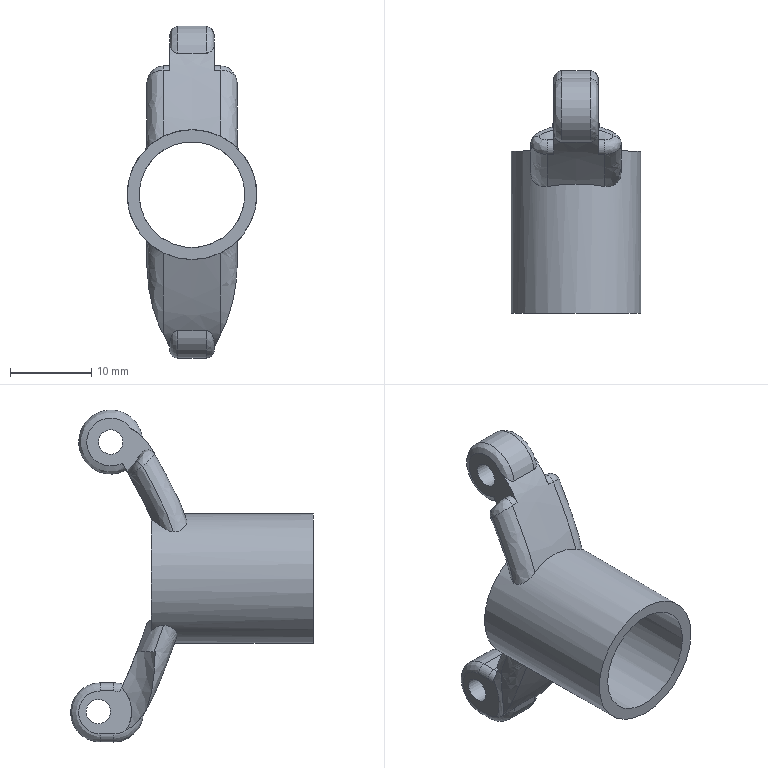Part | STEP file | Wytnij-wyci_gni_cie8 | 1 solid | 57 faces | box 16 x 29.947 x 40.939 mm | volume 2434 mm3 | spline 26 | cylinder 21 | plane 10 | commonest cylinder face diameters 2 x6 7.294 x4 7.918 x4 8.244 x3 3 x2 13.05 x1